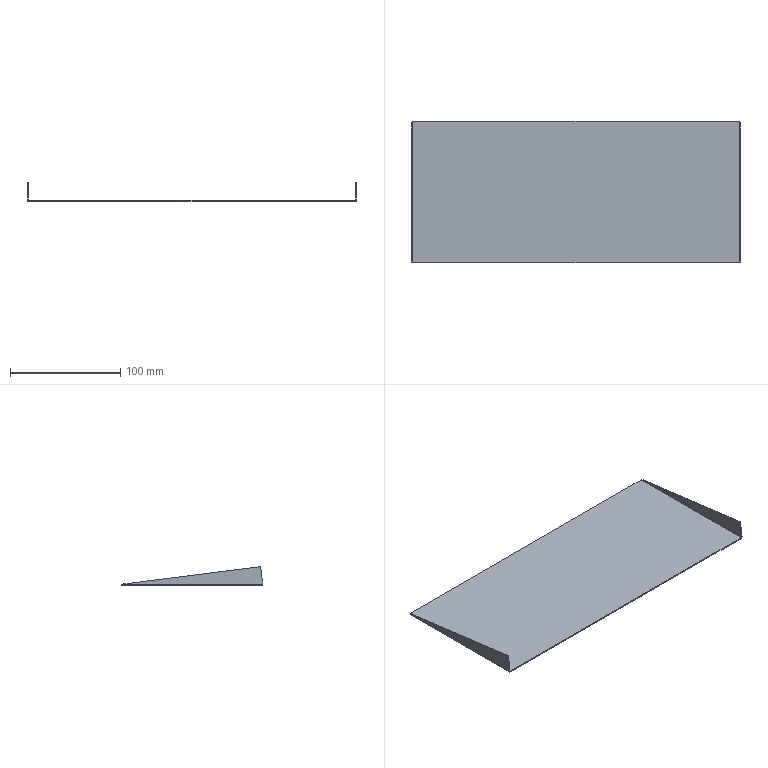Part | SolidWorks | features EdgeFlange 1, FlatPattern 1, MirrorPattern 1, SMBaseFlange 1, SheetMetal 1 | 1 solid | 20 faces | box 299 x 128.5 x 17 mm | volume 40399 mm3 | plane 12 | spline 4 | cylinder 4 | commonest cylinder face diameters 0.4 x2 2.4 x2
STEP:
#1=CARTESIAN_POINT('',(148.3,64.25,-1.));
#2=VERTEX_POINT('',#1);
#3=CARTESIAN_POINT('',(148.3,-64.25,-1.));
#4=VERTEX_POINT('',#3);
#5=CARTESIAN_POINT('',(148.3,64.25,-1.));
#6=DIRECTION('',(0.,-1.,0.));
#7=VECTOR('',#6,1000.);
#8=LINE('',#5,#7);
#9=EDGE_CURVE('',#2,#4,#8,.T.);
#10=ORIENTED_EDGE('',*,*,#9,.T.);
#11=CARTESIAN_POINT('',(-148.3,-64.25,-1.));
#12=VERTEX_POINT('',#11);
#13=CARTESIAN_POINT('',(-149.5,-64.25,-1.));
#14=DIRECTION('',(1.,0.,0.));
#15=VECTOR('',#14,1000.);
#16=LINE('',#13,#15);
#17=EDGE_CURVE('',#12,#4,#16,.T.);
#18=ORIENTED_EDGE('',*,*,#17,.F.);
#19=CARTESIAN_POINT('',(-148.3,64.25,-1.));
#20=VERTEX_POINT('',#19);
#21=CARTESIAN_POINT('',(-148.3,-64.25,-1.));
#22=DIRECTION('',(0.,1.,0.));
#23=VECTOR('',#22,1000.);
#24=LINE('',#21,#23);
#25=EDGE_CURVE('',#12,#20,#24,.T.);
#26=ORIENTED_EDGE('',*,*,#25,.T.);
#27=CARTESIAN_POINT('',(-149.5,64.25,-1.));
#28=DIRECTION('',(-1.,0.,0.));
#29=VECTOR('',#28,1000.);
#30=LINE('',#27,#29);
#31=EDGE_CURVE('',#2,#20,#30,.T.);
#32=ORIENTED_EDGE('',*,*,#31,.F.);
#33=EDGE_LOOP('',(#10,#18,#26,#32));
#34=FACE_OUTER_BOUND('',#33,.T.);
#35=CARTESIAN_POINT('',(0.,0.,-1.));
#36=DIRECTION('',(0.,0.,1.));
#37=DIRECTION('',(1.,0.,0.));
#38=AXIS2_PLACEMENT_3D('',#35,#36,#37);
#39=PLANE('',#38);
#40=ADVANCED_FACE('',(#34),#39,.F.);
#41=CARTESIAN_POINT('',(-148.3,-64.25,0.));
#42=VERTEX_POINT('',#41);
#43=CARTESIAN_POINT('',(148.3,-64.25,0.));
#44=VERTEX_POINT('',#43);
#45=CARTESIAN_POINT('',(-149.5,-64.25,0.));
#46=DIRECTION('',(1.,0.,0.));
#47=VECTOR('',#46,1000.);
#48=LINE('',#45,#47);
#49=EDGE_CURVE('',#42,#44,#48,.T.);
#50=ORIENTED_EDGE('',*,*,#49,.T.);
#51=CARTESIAN_POINT('',(148.3,64.25,0.));
#52=VERTEX_POINT('',#51);
#53=CARTESIAN_POINT('',(148.3,64.25,0.));
#54=DIRECTION('',(0.,-1.,0.));
#55=VECTOR('',#54,1000.);
#56=LINE('',#53,#55);
#57=EDGE_CURVE('',#52,#44,#56,.T.);
#58=ORIENTED_EDGE('',*,*,#57,.F.);
#59=CARTESIAN_POINT('',(-148.3,64.25,0.));
#60=VERTEX_POINT('',#59);
#61=CARTESIAN_POINT('',(-149.5,64.25,0.));
#62=DIRECTION('',(-1.,0.,0.));
#63=VECTOR('',#62,1000.);
#64=LINE('',#61,#63);
#65=EDGE_CURVE('',#52,#60,#64,.T.);
#66=ORIENTED_EDGE('',*,*,#65,.T.);
#67=CARTESIAN_POINT('',(-148.3,-64.25,0.));
#68=DIRECTION('',(0.,1.,0.));
#69=VECTOR('',#68,1000.);
#70=LINE('',#67,#69);
#71=EDGE_CURVE('',#42,#60,#70,.T.);
#72=ORIENTED_EDGE('',*,*,#71,.F.);
#73=EDGE_LOOP('',(#50,#58,#66,#72));
#74=FACE_OUTER_BOUND('',#73,.T.);
#75=CARTESIAN_POINT('',(0.,0.,0.));
#76=DIRECTION('',(0.,0.,1.));
#77=DIRECTION('',(1.,0.,0.));
#78=AXIS2_PLACEMENT_3D('',#75,#76,#77);
#79=PLANE('',#78);
#80=ADVANCED_FACE('',(#74),#79,.T.);
#81=ORIENTED_EDGE('',*,*,#65,.F.);
#82=CARTESIAN_POINT('',(148.3,64.25,0.));
#83=DIRECTION('',(0.,0.,-1.));
#84=VECTOR('',#83,1000.);
#85=LINE('',#82,#84);
#86=EDGE_CURVE('',#52,#2,#85,.T.);
#87=ORIENTED_EDGE('',*,*,#86,.T.);
#88=ORIENTED_EDGE('',*,*,#31,.T.);
#89=CARTESIAN_POINT('',(-148.3,64.25,0.));
#90=DIRECTION('',(0.,0.,-1.));
#91=VECTOR('',#90,1000.);
#92=LINE('',#89,#91);
#93=EDGE_CURVE('',#60,#20,#92,.T.);
#94=ORIENTED_EDGE('',*,*,#93,.F.);
#95=EDGE_LOOP('',(#81,#87,#88,#94));
#96=FACE_OUTER_BOUND('',#95,.T.);
#97=CARTESIAN_POINT('',(-149.5,64.25,-1.));
#98=DIRECTION('',(0.,1.,0.));
#99=DIRECTION('',(0.,0.,1.));
#100=AXIS2_PLACEMENT_3D('',#97,#98,#99);
#101=PLANE('',#100);
#102=ADVANCED_FACE('',(#96),#101,.T.);
#103=CARTESIAN_POINT('',(148.3,-64.25,0.));
#104=DIRECTION('',(0.,0.,-1.));
#105=VECTOR('',#104,1000.);
#106=LINE('',#103,#105);
#107=EDGE_CURVE('',#44,#4,#106,.T.);
#108=ORIENTED_EDGE('',*,*,#107,.F.);
#109=ORIENTED_EDGE('',*,*,#49,.F.);
#110=CARTESIAN_POINT('',(-148.3,-64.25,0.));
#111=DIRECTION('',(0.,0.,-1.));
#112=VECTOR('',#111,1000.);
#113=LINE('',#110,#112);
#114=EDGE_CURVE('',#42,#12,#113,.T.);
#115=ORIENTED_EDGE('',*,*,#114,.T.);
#116=ORIENTED_EDGE('',*,*,#17,.T.);
#117=EDGE_LOOP('',(#108,#109,#115,#116));
#118=FACE_OUTER_BOUND('',#117,.T.);
#119=CARTESIAN_POINT('',(-149.5,-64.25,-1.));
#120=DIRECTION('',(0.,-1.,0.));
#121=DIRECTION('',(0.,0.,-1.));
#122=AXIS2_PLACEMENT_3D('',#119,#120,#121);
#123=PLANE('',#122);
#124=ADVANCED_FACE('',(#118),#123,.T.);
#125=CARTESIAN_POINT('',(-148.5,62.669,0.2));
#126=VERTEX_POINT('',#125);
#127=CARTESIAN_POINT('',(-149.5,62.669,0.2));
#128=VERTEX_POINT('',#127);
#129=CARTESIAN_POINT('',(-149.5,62.669,0.2));
#130=DIRECTION('',(-1.,0.,0.));
#131=VECTOR('',#130,1000.);
#132=LINE('',#129,#131);
#133=EDGE_CURVE('',#126,#128,#132,.T.);
#134=ORIENTED_EDGE('',*,*,#133,.F.);
#135=CARTESIAN_POINT('',(-148.3,64.25,0.));
#136=CARTESIAN_POINT('',(-148.352,63.987,0.));
#137=CARTESIAN_POINT('',(-148.404,63.723,0.02155));
#138=CARTESIAN_POINT('',(-148.478,63.196,0.0956));
#139=CARTESIAN_POINT('',(-148.5,62.933,0.1476));
#140=CARTESIAN_POINT('',(-148.5,62.669,0.2));
#141=B_SPLINE_CURVE_WITH_KNOTS('',3,(#135,#136,#137,#138,#139,#140),.UNSPECIFIED.,.F.,.F.,(4,2,4),(0.,0.5,1.),.UNSPECIFIED.);
#142=EDGE_CURVE('',#60,#126,#141,.T.);
#143=ORIENTED_EDGE('',*,*,#142,.F.);
#144=ORIENTED_EDGE('',*,*,#93,.T.);
#145=CARTESIAN_POINT('',(-148.3,64.25,-1.));
#146=CARTESIAN_POINT('',(-148.458,64.117,-1.));
#147=CARTESIAN_POINT('',(-148.613,63.988,-0.9692));
#148=CARTESIAN_POINT('',(-148.904,63.723,-0.8488));
#149=CARTESIAN_POINT('',(-149.036,63.592,-0.7603));
#150=CARTESIAN_POINT('',(-149.259,63.329,-0.5388));
#151=CARTESIAN_POINT('',(-149.348,63.197,-0.4053));
#152=CARTESIAN_POINT('',(-149.468,62.935,-0.1165));
#153=CARTESIAN_POINT('',(-149.5,62.802,0.04158));
#154=CARTESIAN_POINT('',(-149.5,62.669,0.2));
#155=B_SPLINE_CURVE_WITH_KNOTS('',3,(#145,#146,#147,#148,#149,#150,#151,#152,#153,#154),.UNSPECIFIED.,.F.,.F.,(4,2,2,2,4),(0.,0.0006115,0.001223,0.001835,0.002446),.UNSPECIFIED.);
#156=EDGE_CURVE('',#20,#128,#155,.T.);
#157=ORIENTED_EDGE('',*,*,#156,.T.);
#158=EDGE_LOOP('',(#134,#143,#144,#157));
#159=FACE_OUTER_BOUND('',#158,.T.);
#160=CARTESIAN_POINT('',(-148.3,64.25,-1.01));
#161=CARTESIAN_POINT('',(-148.458,64.118,-1.01));
#162=CARTESIAN_POINT('',(-148.617,63.987,-0.9785));
#163=CARTESIAN_POINT('',(-148.909,63.723,-0.8573));
#164=CARTESIAN_POINT('',(-149.044,63.591,-0.7676));
#165=CARTESIAN_POINT('',(-149.268,63.328,-0.5436));
#166=CARTESIAN_POINT('',(-149.357,63.196,-0.4094));
#167=CARTESIAN_POINT('',(-149.479,62.933,-0.1167));
#168=CARTESIAN_POINT('',(-149.51,62.801,0.04159));
#169=CARTESIAN_POINT('',(-149.51,62.669,0.2));
#170=CARTESIAN_POINT('',(-148.3,64.25,-1.));
#171=CARTESIAN_POINT('',(-148.457,64.118,-1.));
#172=CARTESIAN_POINT('',(-148.614,63.987,-0.9688));
#173=CARTESIAN_POINT('',(-148.904,63.723,-0.8485));
#174=CARTESIAN_POINT('',(-149.037,63.591,-0.7596));
#175=CARTESIAN_POINT('',(-149.26,63.328,-0.5375));
#176=CARTESIAN_POINT('',(-149.349,63.196,-0.4043));
#177=CARTESIAN_POINT('',(-149.469,62.933,-0.1141));
#178=CARTESIAN_POINT('',(-149.5,62.801,0.0429));
#179=CARTESIAN_POINT('',(-149.5,62.669,0.2));
#180=CARTESIAN_POINT('',(-148.3,64.25,0.));
#181=CARTESIAN_POINT('',(-148.326,64.118,0.));
#182=CARTESIAN_POINT('',(-148.352,63.987,0.005205));
#183=CARTESIAN_POINT('',(-148.401,63.723,0.02524));
#184=CARTESIAN_POINT('',(-148.423,63.591,0.04007));
#185=CARTESIAN_POINT('',(-148.46,63.328,0.07709));
#186=CARTESIAN_POINT('',(-148.475,63.196,0.09928));
#187=CARTESIAN_POINT('',(-148.495,62.933,0.1477));
#188=CARTESIAN_POINT('',(-148.5,62.801,0.1738));
#189=CARTESIAN_POINT('',(-148.5,62.669,0.2));
#190=B_SPLINE_SURFACE_WITH_KNOTS('',1,3,((#160,#161,#162,#163,#164,#165,#166,#167,#168,#169),(#170,#171,#172,#173,#174,#175,#176,#177,#178,#179),(#180,#181,#182,#183,#184,#185,#186,#187,#188,#189)),.UNSPECIFIED.,.F.,.F.,.F.,(2,1,2),(4,2,2,2,4),(-0.01,0.,1.),(0.,0.25,0.5,0.75,1.),.UNSPECIFIED.);
#191=ADVANCED_FACE('',(#159),#190,.F.);
#192=CARTESIAN_POINT('',(-148.5,-64.225,0.2));
#193=VERTEX_POINT('',#192);
#194=CARTESIAN_POINT('',(-148.5,-64.225,0.2));
#195=CARTESIAN_POINT('',(-148.5,-64.229,0.1476));
#196=CARTESIAN_POINT('',(-148.478,-64.233,0.0956));
#197=CARTESIAN_POINT('',(-148.404,-64.242,0.02155));
#198=CARTESIAN_POINT('',(-148.352,-64.246,0.));
#199=CARTESIAN_POINT('',(-148.3,-64.25,0.));
#200=B_SPLINE_CURVE_WITH_KNOTS('',3,(#194,#195,#196,#197,#198,#199),.UNSPECIFIED.,.F.,.F.,(4,2,4),(0.,0.5,1.),.UNSPECIFIED.);
#201=EDGE_CURVE('',#193,#42,#200,.T.);
#202=ORIENTED_EDGE('',*,*,#201,.F.);
#203=CARTESIAN_POINT('',(-149.5,-64.225,0.2));
#204=VERTEX_POINT('',#203);
#205=CARTESIAN_POINT('',(-148.5,-64.225,0.2));
#206=DIRECTION('',(-1.,0.,0.));
#207=VECTOR('',#206,1000.);
#208=LINE('',#205,#207);
#209=EDGE_CURVE('',#193,#204,#208,.T.);
#210=ORIENTED_EDGE('',*,*,#209,.T.);
#211=CARTESIAN_POINT('',(-149.5,-64.225,0.2));
#212=CARTESIAN_POINT('',(-149.5,-64.227,0.04292));
#213=CARTESIAN_POINT('',(-149.469,-64.229,-0.1141));
#214=CARTESIAN_POINT('',(-149.349,-64.233,-0.4043));
#215=CARTESIAN_POINT('',(-149.26,-64.235,-0.5375));
#216=CARTESIAN_POINT('',(-149.037,-64.239,-0.7596));
#217=CARTESIAN_POINT('',(-148.904,-64.242,-0.8485));
#218=CARTESIAN_POINT('',(-148.614,-64.246,-0.9688));
#219=CARTESIAN_POINT('',(-148.457,-64.248,-1.));
#220=CARTESIAN_POINT('',(-148.3,-64.25,-1.));
#221=B_SPLINE_CURVE_WITH_KNOTS('',3,(#211,#212,#213,#214,#215,#216,#217,#218,#219,#220),.UNSPECIFIED.,.F.,.F.,(4,2,2,2,4),(0.,0.25,0.5,0.75,1.),.UNSPECIFIED.);
#222=EDGE_CURVE('',#204,#12,#221,.T.);
#223=ORIENTED_EDGE('',*,*,#222,.T.);
#224=ORIENTED_EDGE('',*,*,#114,.F.);
#225=EDGE_LOOP('',(#202,#210,#223,#224));
#226=FACE_OUTER_BOUND('',#225,.T.);
#227=CARTESIAN_POINT('',(-149.51,-64.225,0.2));
#228=CARTESIAN_POINT('',(-149.51,-64.227,0.04158));
#229=CARTESIAN_POINT('',(-149.479,-64.229,-0.1167));
#230=CARTESIAN_POINT('',(-149.357,-64.233,-0.4094));
#231=CARTESIAN_POINT('',(-149.268,-64.235,-0.5436));
#232=CARTESIAN_POINT('',(-149.044,-64.239,-0.7676));
#233=CARTESIAN_POINT('',(-148.909,-64.242,-0.8573));
#234=CARTESIAN_POINT('',(-148.617,-64.246,-0.9785));
#235=CARTESIAN_POINT('',(-148.458,-64.248,-1.01));
#236=CARTESIAN_POINT('',(-148.3,-64.25,-1.01));
#237=CARTESIAN_POINT('',(-149.5,-64.225,0.2));
#238=CARTESIAN_POINT('',(-149.5,-64.227,0.04289));
#239=CARTESIAN_POINT('',(-149.469,-64.229,-0.1141));
#240=CARTESIAN_POINT('',(-149.349,-64.233,-0.4043));
#241=CARTESIAN_POINT('',(-149.26,-64.235,-0.5375));
#242=CARTESIAN_POINT('',(-149.037,-64.239,-0.7596));
#243=CARTESIAN_POINT('',(-148.904,-64.242,-0.8485));
#244=CARTESIAN_POINT('',(-148.614,-64.246,-0.9688));
#245=CARTESIAN_POINT('',(-148.457,-64.248,-1.));
#246=CARTESIAN_POINT('',(-148.3,-64.25,-1.));
#247=CARTESIAN_POINT('',(-148.5,-64.225,0.2));
#248=CARTESIAN_POINT('',(-148.5,-64.227,0.1738));
#249=CARTESIAN_POINT('',(-148.495,-64.229,0.1477));
#250=CARTESIAN_POINT('',(-148.475,-64.233,0.09928));
#251=CARTESIAN_POINT('',(-148.46,-64.235,0.07709));
#252=CARTESIAN_POINT('',(-148.423,-64.239,0.04007));
#253=CARTESIAN_POINT('',(-148.401,-64.242,0.02524));
#254=CARTESIAN_POINT('',(-148.352,-64.246,0.005205));
#255=CARTESIAN_POINT('',(-148.326,-64.248,0.));
#256=CARTESIAN_POINT('',(-148.3,-64.25,0.));
#257=CARTESIAN_POINT('',(-148.49,-64.225,0.2));
#258=CARTESIAN_POINT('',(-148.49,-64.227,0.1751));
#259=CARTESIAN_POINT('',(-148.485,-64.229,0.1503));
#260=CARTESIAN_POINT('',(-148.466,-64.233,0.1044));
#261=CARTESIAN_POINT('',(-148.452,-64.235,0.0833));
#262=CARTESIAN_POINT('',(-148.417,-64.239,0.04814));
#263=CARTESIAN_POINT('',(-148.396,-64.242,0.03407));
#264=CARTESIAN_POINT('',(-148.35,-64.246,0.01504));
#265=CARTESIAN_POINT('',(-148.325,-64.248,0.0101));
#266=CARTESIAN_POINT('',(-148.3,-64.25,0.0101));
#267=B_SPLINE_SURFACE_WITH_KNOTS('',1,3,((#227,#228,#229,#230,#231,#232,#233,#234,#235,#236),(#237,#238,#239,#240,#241,#242,#243,#244,#245,#246),(#247,#248,#249,#250,#251,#252,#253,#254,#255,#256),(#257,#258,#259,#260,#261,#262,#263,#264,#265,#266)),.UNSPECIFIED.,.F.,.F.,.F.,(2,1,1,2),(4,2,2,2,4),(-0.01,0.,1.,1.01),(0.,0.25,0.5,0.75,1.),.UNSPECIFIED.);
#268=ADVANCED_FACE('',(#226),#267,.F.);
#269=ORIENTED_EDGE('',*,*,#25,.F.);
#270=ORIENTED_EDGE('',*,*,#222,.F.);
#271=CARTESIAN_POINT('',(-149.5,62.669,0.2));
#272=DIRECTION('',(0.,1.,0.));
#273=VECTOR('',#272,1000.);
#274=LINE('',#271,#273);
#275=EDGE_CURVE('',#204,#128,#274,.T.);
#276=ORIENTED_EDGE('',*,*,#275,.T.);
#277=ORIENTED_EDGE('',*,*,#156,.F.);
#278=EDGE_LOOP('',(#269,#270,#276,#277));
#279=FACE_OUTER_BOUND('',#278,.T.);
#280=CARTESIAN_POINT('',(-148.3,-64.25,0.2));
#281=DIRECTION('',(0.,-1.,0.));
#282=DIRECTION('',(-1.,0.,0.));
#283=AXIS2_PLACEMENT_3D('',#280,#281,#282);
#284=CYLINDRICAL_SURFACE('',#283,1.2);
#285=ADVANCED_FACE('',(#279),#284,.T.);
#286=ORIENTED_EDGE('',*,*,#71,.T.);
#287=ORIENTED_EDGE('',*,*,#142,.T.);
#288=CARTESIAN_POINT('',(-148.5,62.669,0.2));
#289=DIRECTION('',(0.,-1.,0.));
#290=VECTOR('',#289,1000.);
#291=LINE('',#288,#290);
#292=EDGE_CURVE('',#126,#193,#291,.T.);
#293=ORIENTED_EDGE('',*,*,#292,.T.);
#294=ORIENTED_EDGE('',*,*,#201,.T.);
#295=EDGE_LOOP('',(#286,#287,#293,#294));
#296=FACE_OUTER_BOUND('',#295,.T.);
#297=CARTESIAN_POINT('',(-148.3,-64.25,0.2));
#298=DIRECTION('',(0.,-1.,0.));
#299=DIRECTION('',(-1.,0.,0.));
#300=AXIS2_PLACEMENT_3D('',#297,#298,#299);
#301=CYLINDRICAL_SURFACE('',#300,0.2);
#302=ADVANCED_FACE('',(#296),#301,.F.);
#303=ORIENTED_EDGE('',*,*,#133,.T.);
#304=CARTESIAN_POINT('',(-149.5,-62.226,16.));
#305=VERTEX_POINT('',#304);
#306=CARTESIAN_POINT('',(-149.5,1.012,8.));
#307=DIRECTION('',(0.,0.9921,-0.1255));
#308=VECTOR('',#307,1000.);
#309=LINE('',#306,#308);
#310=EDGE_CURVE('',#305,#128,#309,.T.);
#311=ORIENTED_EDGE('',*,*,#310,.F.);
#312=CARTESIAN_POINT('',(-148.5,-62.226,16.));
#313=VERTEX_POINT('',#312);
#314=CARTESIAN_POINT('',(-149.5,-62.226,16.));
#315=DIRECTION('',(1.,0.,0.));
#316=VECTOR('',#315,1000.);
#317=LINE('',#314,#316);
#318=EDGE_CURVE('',#305,#313,#317,.T.);
#319=ORIENTED_EDGE('',*,*,#318,.T.);
#320=CARTESIAN_POINT('',(-148.5,-62.226,16.));
#321=DIRECTION('',(0.,0.9921,-0.1255));
#322=VECTOR('',#321,1000.);
#323=LINE('',#320,#322);
#324=EDGE_CURVE('',#313,#126,#323,.T.);
#325=ORIENTED_EDGE('',*,*,#324,.T.);
#326=EDGE_LOOP('',(#303,#311,#319,#325));
#327=FACE_OUTER_BOUND('',#326,.T.);
#328=CARTESIAN_POINT('',(-149.5,-62.226,16.));
#329=DIRECTION('',(0.,-0.1255,-0.9921));
#330=DIRECTION('',(0.,0.9921,-0.1255));
#331=AXIS2_PLACEMENT_3D('',#328,#329,#330);
#332=PLANE('',#331);
#333=ADVANCED_FACE('',(#327),#332,.F.);
#334=ORIENTED_EDGE('',*,*,#209,.F.);
#335=CARTESIAN_POINT('',(-148.5,-64.25,0.));
#336=DIRECTION('',(0.,0.1255,0.9921));
#337=VECTOR('',#336,1000.);
#338=LINE('',#335,#337);
#339=EDGE_CURVE('',#193,#313,#338,.T.);
#340=ORIENTED_EDGE('',*,*,#339,.T.);
#341=ORIENTED_EDGE('',*,*,#318,.F.);
#342=CARTESIAN_POINT('',(-149.5,-63.238,8.));
#343=DIRECTION('',(0.,0.1255,0.9921));
#344=VECTOR('',#343,1000.);
#345=LINE('',#342,#344);
#346=EDGE_CURVE('',#204,#305,#345,.T.);
#347=ORIENTED_EDGE('',*,*,#346,.F.);
#348=EDGE_LOOP('',(#334,#340,#341,#347));
#349=FACE_OUTER_BOUND('',#348,.T.);
#350=CARTESIAN_POINT('',(-149.5,-64.25,0.));
#351=DIRECTION('',(0.,0.9921,-0.1255));
#352=DIRECTION('',(0.,0.1255,0.9921));
#353=AXIS2_PLACEMENT_3D('',#350,#351,#352);
#354=PLANE('',#353);
#355=ADVANCED_FACE('',(#349),#354,.F.);
#356=ORIENTED_EDGE('',*,*,#275,.F.);
#357=ORIENTED_EDGE('',*,*,#346,.T.);
#358=ORIENTED_EDGE('',*,*,#310,.T.);
#359=EDGE_LOOP('',(#356,#357,#358));
#360=FACE_OUTER_BOUND('',#359,.T.);
#361=CARTESIAN_POINT('',(-149.5,0.,0.));
#362=DIRECTION('',(1.,0.,0.));
#363=DIRECTION('',(0.,0.,-1.));
#364=AXIS2_PLACEMENT_3D('',#361,#362,#363);
#365=PLANE('',#364);
#366=ADVANCED_FACE('',(#360),#365,.F.);
#367=ORIENTED_EDGE('',*,*,#339,.F.);
#368=ORIENTED_EDGE('',*,*,#292,.F.);
#369=ORIENTED_EDGE('',*,*,#324,.F.);
#370=EDGE_LOOP('',(#367,#368,#369));
#371=FACE_OUTER_BOUND('',#370,.T.);
#372=CARTESIAN_POINT('',(-148.5,0.,0.));
#373=DIRECTION('',(1.,0.,0.));
#374=DIRECTION('',(0.,0.,-1.));
#375=AXIS2_PLACEMENT_3D('',#372,#373,#374);
#376=PLANE('',#375);
#377=ADVANCED_FACE('',(#371),#376,.T.);
#378=CARTESIAN_POINT('',(148.5,-64.225,0.2));
#379=VERTEX_POINT('',#378);
#380=CARTESIAN_POINT('',(149.5,-64.225,0.2));
#381=VERTEX_POINT('',#380);
#382=CARTESIAN_POINT('',(149.5,-64.225,0.2));
#383=DIRECTION('',(1.,0.,0.));
#384=VECTOR('',#383,1000.);
#385=LINE('',#382,#384);
#386=EDGE_CURVE('',#379,#381,#385,.T.);
#387=ORIENTED_EDGE('',*,*,#386,.F.);
#388=CARTESIAN_POINT('',(148.3,-64.25,0.));
#389=CARTESIAN_POINT('',(148.352,-64.246,0.));
#390=CARTESIAN_POINT('',(148.404,-64.242,0.02155));
#391=CARTESIAN_POINT('',(148.478,-64.233,0.0956));
#392=CARTESIAN_POINT('',(148.5,-64.229,0.1476));
#393=CARTESIAN_POINT('',(148.5,-64.225,0.2));
#394=B_SPLINE_CURVE_WITH_KNOTS('',3,(#388,#389,#390,#391,#392,#393),.UNSPECIFIED.,.F.,.F.,(4,2,4),(0.,0.5,1.),.UNSPECIFIED.);
#395=EDGE_CURVE('',#44,#379,#394,.T.);
#396=ORIENTED_EDGE('',*,*,#395,.F.);
#397=ORIENTED_EDGE('',*,*,#107,.T.);
#398=CARTESIAN_POINT('',(148.3,-64.25,-1.));
#399=CARTESIAN_POINT('',(148.457,-64.248,-1.));
#400=CARTESIAN_POINT('',(148.614,-64.246,-0.9688));
#401=CARTESIAN_POINT('',(148.904,-64.242,-0.8485));
#402=CARTESIAN_POINT('',(149.037,-64.239,-0.7596));
#403=CARTESIAN_POINT('',(149.26,-64.235,-0.5375));
#404=CARTESIAN_POINT('',(149.349,-64.233,-0.4043));
#405=CARTESIAN_POINT('',(149.469,-64.229,-0.1141));
#406=CARTESIAN_POINT('',(149.5,-64.227,0.04292));
#407=CARTESIAN_POINT('',(149.5,-64.225,0.2));
#408=B_SPLINE_CURVE_WITH_KNOTS('',3,(#398,#399,#400,#401,#402,#403,#404,#405,#406,#407),.UNSPECIFIED.,.F.,.F.,(4,2,2,2,4),(0.,0.25,0.5,0.75,1.),.UNSPECIFIED.);
#409=EDGE_CURVE('',#4,#381,#408,.T.);
#410=ORIENTED_EDGE('',*,*,#409,.T.);
#411=EDGE_LOOP('',(#387,#396,#397,#410));
#412=FACE_OUTER_BOUND('',#411,.T.);
#413=CARTESIAN_POINT('',(148.3,-64.25,-1.01));
#414=CARTESIAN_POINT('',(148.458,-64.248,-1.01));
#415=CARTESIAN_POINT('',(148.617,-64.246,-0.9785));
#416=CARTESIAN_POINT('',(148.909,-64.242,-0.8573));
#417=CARTESIAN_POINT('',(149.044,-64.239,-0.7676));
#418=CARTESIAN_POINT('',(149.268,-64.235,-0.5436));
#419=CARTESIAN_POINT('',(149.357,-64.233,-0.4094));
#420=CARTESIAN_POINT('',(149.479,-64.229,-0.1167));
#421=CARTESIAN_POINT('',(149.51,-64.227,0.04158));
#422=CARTESIAN_POINT('',(149.51,-64.225,0.2));
#423=CARTESIAN_POINT('',(148.3,-64.25,-1.));
#424=CARTESIAN_POINT('',(148.457,-64.248,-1.));
#425=CARTESIAN_POINT('',(148.614,-64.246,-0.9688));
#426=CARTESIAN_POINT('',(148.904,-64.242,-0.8485));
#427=CARTESIAN_POINT('',(149.037,-64.239,-0.7596));
#428=CARTESIAN_POINT('',(149.26,-64.235,-0.5375));
#429=CARTESIAN_POINT('',(149.349,-64.233,-0.4043));
#430=CARTESIAN_POINT('',(149.469,-64.229,-0.1141));
#431=CARTESIAN_POINT('',(149.5,-64.227,0.04289));
#432=CARTESIAN_POINT('',(149.5,-64.225,0.2));
#433=CARTESIAN_POINT('',(148.3,-64.25,0.));
#434=CARTESIAN_POINT('',(148.326,-64.248,0.));
#435=CARTESIAN_POINT('',(148.352,-64.246,0.005205));
#436=CARTESIAN_POINT('',(148.401,-64.242,0.02524));
#437=CARTESIAN_POINT('',(148.423,-64.239,0.04007));
#438=CARTESIAN_POINT('',(148.46,-64.235,0.07709));
#439=CARTESIAN_POINT('',(148.475,-64.233,0.09928));
#440=CARTESIAN_POINT('',(148.495,-64.229,0.1477));
#441=CARTESIAN_POINT('',(148.5,-64.227,0.1738));
#442=CARTESIAN_POINT('',(148.5,-64.225,0.2));
#443=CARTESIAN_POINT('',(148.3,-64.25,0.0101));
#444=CARTESIAN_POINT('',(148.325,-64.248,0.0101));
#445=CARTESIAN_POINT('',(148.35,-64.246,0.01504));
#446=CARTESIAN_POINT('',(148.396,-64.242,0.03407));
#447=CARTESIAN_POINT('',(148.417,-64.239,0.04814));
#448=CARTESIAN_POINT('',(148.452,-64.235,0.0833));
#449=CARTESIAN_POINT('',(148.466,-64.233,0.1044));
#450=CARTESIAN_POINT('',(148.485,-64.229,0.1503));
#451=CARTESIAN_POINT('',(148.49,-64.227,0.1751));
#452=CARTESIAN_POINT('',(148.49,-64.225,0.2));
#453=B_SPLINE_SURFACE_WITH_KNOTS('',1,3,((#413,#414,#415,#416,#417,#418,#419,#420,#421,#422),(#423,#424,#425,#426,#427,#428,#429,#430,#431,#432),(#433,#434,#435,#436,#437,#438,#439,#440,#441,#442),(#443,#444,#445,#446,#447,#448,#449,#450,#451,#452)),.UNSPECIFIED.,.F.,.F.,.F.,(2,1,1,2),(4,2,2,2,4),(-0.01,0.,1.,1.01),(0.,0.25,0.5,0.75,1.),.UNSPECIFIED.);
#454=ADVANCED_FACE('',(#412),#453,.F.);
#455=CARTESIAN_POINT('',(148.5,62.669,0.2));
#456=VERTEX_POINT('',#455);
#457=CARTESIAN_POINT('',(148.5,62.669,0.2));
#458=CARTESIAN_POINT('',(148.5,62.933,0.1476));
#459=CARTESIAN_POINT('',(148.478,63.196,0.0956));
#460=CARTESIAN_POINT('',(148.404,63.723,0.02155));
#461=CARTESIAN_POINT('',(148.352,63.987,0.));
#462=CARTESIAN_POINT('',(148.3,64.25,0.));
#463=B_SPLINE_CURVE_WITH_KNOTS('',3,(#457,#458,#459,#460,#461,#462),.UNSPECIFIED.,.F.,.F.,(4,2,4),(0.,0.5,1.),.UNSPECIFIED.);
#464=EDGE_CURVE('',#456,#52,#463,.T.);
#465=ORIENTED_EDGE('',*,*,#464,.F.);
#466=CARTESIAN_POINT('',(149.5,62.669,0.2));
#467=VERTEX_POINT('',#466);
#468=CARTESIAN_POINT('',(148.5,62.669,0.2));
#469=DIRECTION('',(1.,0.,0.));
#470=VECTOR('',#469,1000.);
#471=LINE('',#468,#470);
#472=EDGE_CURVE('',#456,#467,#471,.T.);
#473=ORIENTED_EDGE('',*,*,#472,.T.);
#474=CARTESIAN_POINT('',(149.5,62.669,0.2));
#475=CARTESIAN_POINT('',(149.5,62.802,0.04158));
#476=CARTESIAN_POINT('',(149.469,62.931,-0.1128));
#477=CARTESIAN_POINT('',(149.349,63.196,-0.404));
#478=CARTESIAN_POINT('',(149.26,63.327,-0.5365));
#479=CARTESIAN_POINT('',(149.039,63.59,-0.7586));
#480=CARTESIAN_POINT('',(148.905,63.722,-0.8479));
#481=CARTESIAN_POINT('',(148.616,63.984,-0.968));
#482=CARTESIAN_POINT('',(148.458,64.117,-1.));
#483=CARTESIAN_POINT('',(148.3,64.25,-1.));
#484=B_SPLINE_CURVE_WITH_KNOTS('',3,(#474,#475,#476,#477,#478,#479,#480,#481,#482,#483),.UNSPECIFIED.,.F.,.F.,(4,2,2,2,4),(0.,0.0006115,0.001223,0.001835,0.002446),.UNSPECIFIED.);
#485=EDGE_CURVE('',#467,#2,#484,.T.);
#486=ORIENTED_EDGE('',*,*,#485,.T.);
#487=ORIENTED_EDGE('',*,*,#86,.F.);
#488=EDGE_LOOP('',(#465,#473,#486,#487));
#489=FACE_OUTER_BOUND('',#488,.T.);
#490=CARTESIAN_POINT('',(149.51,62.669,0.2));
#491=CARTESIAN_POINT('',(149.51,62.801,0.04159));
#492=CARTESIAN_POINT('',(149.479,62.933,-0.1167));
#493=CARTESIAN_POINT('',(149.357,63.196,-0.4094));
#494=CARTESIAN_POINT('',(149.268,63.328,-0.5436));
#495=CARTESIAN_POINT('',(149.044,63.591,-0.7676));
#496=CARTESIAN_POINT('',(148.909,63.723,-0.8573));
#497=CARTESIAN_POINT('',(148.617,63.987,-0.9785));
#498=CARTESIAN_POINT('',(148.458,64.118,-1.01));
#499=CARTESIAN_POINT('',(148.3,64.25,-1.01));
#500=CARTESIAN_POINT('',(149.5,62.669,0.2));
#501=CARTESIAN_POINT('',(149.5,62.801,0.0429));
#502=CARTESIAN_POINT('',(149.469,62.933,-0.1141));
#503=CARTESIAN_POINT('',(149.349,63.196,-0.4043));
#504=CARTESIAN_POINT('',(149.26,63.328,-0.5375));
#505=CARTESIAN_POINT('',(149.037,63.591,-0.7596));
#506=CARTESIAN_POINT('',(148.904,63.723,-0.8485));
#507=CARTESIAN_POINT('',(148.614,63.987,-0.9688));
#508=CARTESIAN_POINT('',(148.457,64.118,-1.));
#509=CARTESIAN_POINT('',(148.3,64.25,-1.));
#510=CARTESIAN_POINT('',(148.5,62.669,0.2));
#511=CARTESIAN_POINT('',(148.5,62.801,0.1738));
#512=CARTESIAN_POINT('',(148.495,62.933,0.1477));
#513=CARTESIAN_POINT('',(148.475,63.196,0.09928));
#514=CARTESIAN_POINT('',(148.46,63.328,0.07709));
#515=CARTESIAN_POINT('',(148.423,63.591,0.04007));
#516=CARTESIAN_POINT('',(148.401,63.723,0.02524));
#517=CARTESIAN_POINT('',(148.352,63.987,0.005205));
#518=CARTESIAN_POINT('',(148.326,64.118,0.));
#519=CARTESIAN_POINT('',(148.3,64.25,0.));
#520=B_SPLINE_SURFACE_WITH_KNOTS('',1,3,((#490,#491,#492,#493,#494,#495,#496,#497,#498,#499),(#500,#501,#502,#503,#504,#505,#506,#507,#508,#509),(#510,#511,#512,#513,#514,#515,#516,#517,#518,#519)),.UNSPECIFIED.,.F.,.F.,.F.,(2,1,2),(4,2,2,2,4),(-0.01,0.,1.),(0.,0.25,0.5,0.75,1.),.UNSPECIFIED.);
#521=ADVANCED_FACE('',(#489),#520,.F.);
#522=ORIENTED_EDGE('',*,*,#9,.F.);
#523=ORIENTED_EDGE('',*,*,#485,.F.);
#524=CARTESIAN_POINT('',(149.5,-64.225,0.2));
#525=DIRECTION('',(0.,-1.,0.));
#526=VECTOR('',#525,1000.);
#527=LINE('',#524,#526);
#528=EDGE_CURVE('',#467,#381,#527,.T.);
#529=ORIENTED_EDGE('',*,*,#528,.T.);
#530=ORIENTED_EDGE('',*,*,#409,.F.);
#531=EDGE_LOOP('',(#522,#523,#529,#530));
#532=FACE_OUTER_BOUND('',#531,.T.);
#533=CARTESIAN_POINT('',(148.3,64.25,0.2));
#534=DIRECTION('',(0.,1.,0.));
#535=DIRECTION('',(1.,0.,0.));
#536=AXIS2_PLACEMENT_3D('',#533,#534,#535);
#537=CYLINDRICAL_SURFACE('',#536,1.2);
#538=ADVANCED_FACE('',(#532),#537,.T.);
#539=ORIENTED_EDGE('',*,*,#57,.T.);
#540=ORIENTED_EDGE('',*,*,#395,.T.);
#541=CARTESIAN_POINT('',(148.5,-64.225,0.2));
#542=DIRECTION('',(0.,1.,0.));
#543=VECTOR('',#542,1000.);
#544=LINE('',#541,#543);
#545=EDGE_CURVE('',#379,#456,#544,.T.);
#546=ORIENTED_EDGE('',*,*,#545,.T.);
#547=ORIENTED_EDGE('',*,*,#464,.T.);
#548=EDGE_LOOP('',(#539,#540,#546,#547));
#549=FACE_OUTER_BOUND('',#548,.T.);
#550=CARTESIAN_POINT('',(148.3,64.25,0.2));
#551=DIRECTION('',(0.,1.,0.));
#552=DIRECTION('',(1.,0.,0.));
#553=AXIS2_PLACEMENT_3D('',#550,#551,#552);
#554=CYLINDRICAL_SURFACE('',#553,0.2);
#555=ADVANCED_FACE('',(#549),#554,.F.);
#556=CARTESIAN_POINT('',(149.5,-62.226,16.));
#557=VERTEX_POINT('',#556);
#558=CARTESIAN_POINT('',(149.5,-62.226,16.));
#559=DIRECTION('',(0.,0.9921,-0.1255));
#560=VECTOR('',#559,1000.);
#561=LINE('',#558,#560);
#562=EDGE_CURVE('',#557,#467,#561,.T.);
#563=ORIENTED_EDGE('',*,*,#562,.T.);
#564=ORIENTED_EDGE('',*,*,#472,.F.);
#565=CARTESIAN_POINT('',(148.5,-62.226,16.));
#566=VERTEX_POINT('',#565);
#567=CARTESIAN_POINT('',(148.5,1.012,8.));
#568=DIRECTION('',(0.,0.9921,-0.1255));
#569=VECTOR('',#568,1000.);
#570=LINE('',#567,#569);
#571=EDGE_CURVE('',#566,#456,#570,.T.);
#572=ORIENTED_EDGE('',*,*,#571,.F.);
#573=CARTESIAN_POINT('',(149.5,-62.226,16.));
#574=DIRECTION('',(-1.,0.,0.));
#575=VECTOR('',#574,1000.);
#576=LINE('',#573,#575);
#577=EDGE_CURVE('',#557,#566,#576,.T.);
#578=ORIENTED_EDGE('',*,*,#577,.F.);
#579=EDGE_LOOP('',(#563,#564,#572,#578));
#580=FACE_OUTER_BOUND('',#579,.T.);
#581=CARTESIAN_POINT('',(149.5,-62.226,16.));
#582=DIRECTION('',(0.,0.1255,0.9921));
#583=DIRECTION('',(0.,-0.9921,0.1255));
#584=AXIS2_PLACEMENT_3D('',#581,#582,#583);
#585=PLANE('',#584);
#586=ADVANCED_FACE('',(#580),#585,.T.);
#587=CARTESIAN_POINT('',(148.5,-63.238,8.));
#588=DIRECTION('',(0.,0.1255,0.9921));
#589=VECTOR('',#588,1000.);
#590=LINE('',#587,#589);
#591=EDGE_CURVE('',#379,#566,#590,.T.);
#592=ORIENTED_EDGE('',*,*,#591,.F.);
#593=ORIENTED_EDGE('',*,*,#386,.T.);
#594=CARTESIAN_POINT('',(149.5,-64.25,0.));
#595=DIRECTION('',(0.,0.1255,0.9921));
#596=VECTOR('',#595,1000.);
#597=LINE('',#594,#596);
#598=EDGE_CURVE('',#381,#557,#597,.T.);
#599=ORIENTED_EDGE('',*,*,#598,.T.);
#600=ORIENTED_EDGE('',*,*,#577,.T.);
#601=EDGE_LOOP('',(#592,#593,#599,#600));
#602=FACE_OUTER_BOUND('',#601,.T.);
#603=CARTESIAN_POINT('',(149.5,-64.25,0.));
#604=DIRECTION('',(0.,-0.9921,0.1255));
#605=DIRECTION('',(0.,-0.1255,-0.9921));
#606=AXIS2_PLACEMENT_3D('',#603,#604,#605);
#607=PLANE('',#606);
#608=ADVANCED_FACE('',(#602),#607,.T.);
#609=ORIENTED_EDGE('',*,*,#528,.F.);
#610=ORIENTED_EDGE('',*,*,#562,.F.);
#611=ORIENTED_EDGE('',*,*,#598,.F.);
#612=EDGE_LOOP('',(#609,#610,#611));
#613=FACE_OUTER_BOUND('',#612,.T.);
#614=CARTESIAN_POINT('',(149.5,0.,0.));
#615=DIRECTION('',(-1.,0.,0.));
#616=DIRECTION('',(0.,0.,-1.));
#617=AXIS2_PLACEMENT_3D('',#614,#615,#616);
#618=PLANE('',#617);
#619=ADVANCED_FACE('',(#613),#618,.F.);
#620=ORIENTED_EDGE('',*,*,#571,.T.);
#621=ORIENTED_EDGE('',*,*,#545,.F.);
#622=ORIENTED_EDGE('',*,*,#591,.T.);
#623=EDGE_LOOP('',(#620,#621,#622));
#624=FACE_OUTER_BOUND('',#623,.T.);
#625=CARTESIAN_POINT('',(148.5,0.,0.));
#626=DIRECTION('',(-1.,0.,0.));
#627=DIRECTION('',(0.,0.,-1.));
#628=AXIS2_PLACEMENT_3D('',#625,#626,#627);
#629=PLANE('',#628);
#630=ADVANCED_FACE('',(#624),#629,.T.);
#631=CLOSED_SHELL('',(#40,#80,#102,#124,#191,#268,#285,#302,#333,#355,#366,#377,#454,#521,#538,#555,#586,#608,#619,#630));
#632=MANIFOLD_SOLID_BREP('',#631);
#633=CARTESIAN_POINT('',(0.,0.,0.));
#634=DIRECTION('',(0.,0.,1.));
#635=DIRECTION('',(1.,0.,0.));
#636=AXIS2_PLACEMENT_3D('',#633,#634,#635);
#637=(LENGTH_UNIT()NAMED_UNIT(*)SI_UNIT(.MILLI.,.METRE.));
#638=UNCERTAINTY_MEASURE_WITH_UNIT(LENGTH_MEASURE(0.00001),#637,'','');
#639=(NAMED_UNIT(*)PLANE_ANGLE_UNIT()SI_UNIT($,.RADIAN.));
#640=(NAMED_UNIT(*)SI_UNIT($,.STERADIAN.)SOLID_ANGLE_UNIT());
#641=(GEOMETRIC_REPRESENTATION_CONTEXT(3)GLOBAL_UNCERTAINTY_ASSIGNED_CONTEXT((#638))GLOBAL_UNIT_ASSIGNED_CONTEXT((#637,#639,#640))REPRESENTATION_CONTEXT('',''));
#642=ADVANCED_BREP_SHAPE_REPRESENTATION('',(#632,#636),#641);